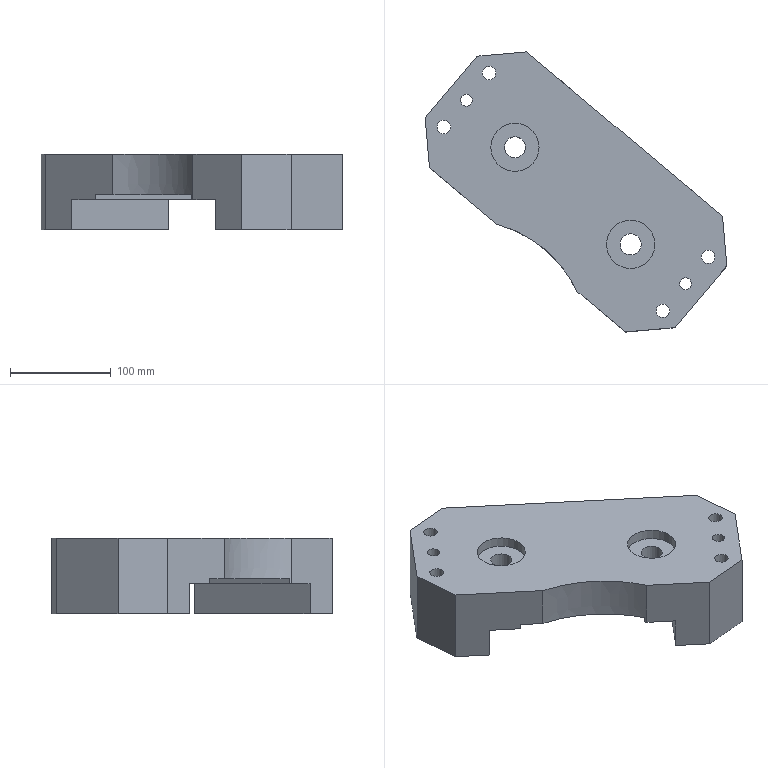Part | NX | features solid 2 | 1 solid | 52 faces | box 299.621 x 278.175 x 75 mm | volume 2327315 mm3 | plane 25 | cylinder 20 | cone 6 | spline 1 | commonest cylinder face diameters 10.579 x4 12 x4 13.5 x4 19.5 x4 21 x2 48 x2
STEP:
#1=CARTESIAN_POINT('',(632.553,521.759,95.));
#2=VERTEX_POINT('',#1);
#3=CARTESIAN_POINT('',(643.053,521.759,95.));
#4=DIRECTION('',(0.,0.,-1.));
#5=DIRECTION('',(-1.,0.,0.));
#6=AXIS2_PLACEMENT_3D('',#3,#4,#5);
#7=CIRCLE('',#6,10.5);
#8=EDGE_CURVE('',#2,#2,#7,.F.);
#9=ORIENTED_EDGE('',*,*,#8,.T.);
#10=EDGE_LOOP('',(#9));
#11=FACE_BOUND('',#10,.T.);
#12=CARTESIAN_POINT('',(588.722,477.235,95.));
#13=VERTEX_POINT('',#12);
#14=CARTESIAN_POINT('',(589.775,475.086,95.));
#15=VERTEX_POINT('',#14);
#16=CARTESIAN_POINT('',(588.722,477.235,95.));
#17=CARTESIAN_POINT('',(589.08,476.522,95.));
#18=CARTESIAN_POINT('',(589.431,475.806,95.));
#19=CARTESIAN_POINT('',(589.775,475.086,95.));
#20=B_SPLINE_CURVE_WITH_KNOTS('',3,(#16,#17,#18,#19),.UNSPECIFIED.,.F.,.F.,(4,4),(0.003786,0.006174),.UNSPECIFIED.);
#21=EDGE_CURVE('',#13,#15,#20,.T.);
#22=ORIENTED_EDGE('',*,*,#21,.F.);
#23=CARTESIAN_POINT('',(684.517,591.399,95.));
#24=VERTEX_POINT('',#23);
#25=CARTESIAN_POINT('',(594.527,484.153,95.));
#26=DIRECTION('',(-0.6428,-0.766,0.));
#27=VECTOR('',#26,1000.);
#28=LINE('',#25,#27);
#29=EDGE_CURVE('',#13,#24,#28,.F.);
#30=ORIENTED_EDGE('',*,*,#29,.T.);
#31=CARTESIAN_POINT('',(708.264,571.473,95.));
#32=VERTEX_POINT('',#31);
#33=CARTESIAN_POINT('',(577.654,681.068,95.));
#34=DIRECTION('',(-0.766,0.6428,0.));
#35=VECTOR('',#34,1000.);
#36=LINE('',#33,#35);
#37=EDGE_CURVE('',#32,#24,#36,.T.);
#38=ORIENTED_EDGE('',*,*,#37,.F.);
#39=CARTESIAN_POINT('',(611.846,456.566,95.));
#40=VERTEX_POINT('',#39);
#41=CARTESIAN_POINT('',(618.274,464.227,95.));
#42=DIRECTION('',(-0.6428,-0.766,0.));
#43=VECTOR('',#42,1000.);
#44=LINE('',#41,#43);
#45=EDGE_CURVE('',#32,#40,#44,.T.);
#46=ORIENTED_EDGE('',*,*,#45,.T.);
#47=CARTESIAN_POINT('',(481.236,566.161,95.));
#48=DIRECTION('',(0.766,-0.6428,0.));
#49=VECTOR('',#48,1000.);
#50=LINE('',#47,#49);
#51=EDGE_CURVE('',#15,#40,#50,.T.);
#52=ORIENTED_EDGE('',*,*,#51,.F.);
#53=EDGE_LOOP('',(#22,#30,#38,#46,#52));
#54=FACE_BOUND('',#53,.T.);
#55=CARTESIAN_POINT('',(487.664,573.822,95.));
#56=DIRECTION('',(0.,0.,1.));
#57=DIRECTION('',(0.08716,-0.9962,0.));
#58=AXIS2_PLACEMENT_3D('',#55,#56,#57);
#59=PLANE('',#58);
#60=ADVANCED_FACE('',(#11,#54),#59,.F.);
#61=CARTESIAN_POINT('',(589.775,475.086,140.));
#62=VERTEX_POINT('',#61);
#63=CARTESIAN_POINT('',(589.775,475.086,87.5));
#64=DIRECTION('',(0.,0.,-1.));
#65=VECTOR('',#64,1000.);
#66=LINE('',#63,#65);
#67=EDGE_CURVE('',#15,#62,#66,.F.);
#68=ORIENTED_EDGE('',*,*,#67,.F.);
#69=ORIENTED_EDGE('',*,*,#51,.T.);
#70=CARTESIAN_POINT('',(611.846,456.566,65.));
#71=VERTEX_POINT('',#70);
#72=CARTESIAN_POINT('',(611.846,456.566,95.));
#73=DIRECTION('',(0.,0.,1.));
#74=VECTOR('',#73,1000.);
#75=LINE('',#72,#74);
#76=EDGE_CURVE('',#71,#40,#75,.T.);
#77=ORIENTED_EDGE('',*,*,#76,.F.);
#78=CARTESIAN_POINT('',(637.892,434.711,65.));
#79=VERTEX_POINT('',#78);
#80=CARTESIAN_POINT('',(481.236,566.161,65.));
#81=DIRECTION('',(0.766,-0.6428,0.));
#82=VECTOR('',#81,1000.);
#83=LINE('',#80,#82);
#84=EDGE_CURVE('',#71,#79,#83,.T.);
#85=ORIENTED_EDGE('',*,*,#84,.T.);
#86=CARTESIAN_POINT('',(637.892,434.711,140.));
#87=VERTEX_POINT('',#86);
#88=CARTESIAN_POINT('',(637.892,434.711,60.));
#89=DIRECTION('',(0.,0.,-1.));
#90=VECTOR('',#89,1000.);
#91=LINE('',#88,#90);
#92=EDGE_CURVE('',#87,#79,#91,.T.);
#93=ORIENTED_EDGE('',*,*,#92,.F.);
#94=CARTESIAN_POINT('',(481.236,566.161,140.));
#95=DIRECTION('',(0.766,-0.6428,0.));
#96=VECTOR('',#95,1000.);
#97=LINE('',#94,#96);
#98=EDGE_CURVE('',#62,#87,#97,.T.);
#99=ORIENTED_EDGE('',*,*,#98,.F.);
#100=EDGE_LOOP('',(#68,#69,#77,#85,#93,#99));
#101=FACE_BOUND('',#100,.T.);
#102=CARTESIAN_POINT('',(481.236,566.161,95.));
#103=DIRECTION('',(0.6428,0.766,0.));
#104=DIRECTION('',(0.766,-0.6428,0.));
#105=AXIS2_PLACEMENT_3D('',#102,#103,#104);
#106=PLANE('',#105);
#107=ADVANCED_FACE('',(#101),#106,.F.);
#108=CARTESIAN_POINT('',(510.282,541.788,140.));
#109=VERTEX_POINT('',#108);
#110=CARTESIAN_POINT('',(510.282,541.788,100.));
#111=VERTEX_POINT('',#110);
#112=CARTESIAN_POINT('',(510.282,541.788,87.5));
#113=DIRECTION('',(0.,0.,-1.));
#114=VECTOR('',#113,1000.);
#115=LINE('',#112,#114);
#116=EDGE_CURVE('',#109,#111,#115,.T.);
#117=ORIENTED_EDGE('',*,*,#116,.F.);
#118=CARTESIAN_POINT('',(443.317,597.979,140.));
#119=VERTEX_POINT('',#118);
#120=CARTESIAN_POINT('',(481.236,566.161,140.));
#121=DIRECTION('',(0.766,-0.6428,0.));
#122=VECTOR('',#121,1000.);
#123=LINE('',#120,#122);
#124=EDGE_CURVE('',#119,#109,#123,.T.);
#125=ORIENTED_EDGE('',*,*,#124,.F.);
#126=CARTESIAN_POINT('',(443.317,597.979,65.));
#127=VERTEX_POINT('',#126);
#128=CARTESIAN_POINT('',(443.317,597.979,95.));
#129=DIRECTION('',(0.,0.,1.));
#130=VECTOR('',#129,1000.);
#131=LINE('',#128,#130);
#132=EDGE_CURVE('',#127,#119,#131,.T.);
#133=ORIENTED_EDGE('',*,*,#132,.F.);
#134=CARTESIAN_POINT('',(469.362,576.125,65.));
#135=VERTEX_POINT('',#134);
#136=CARTESIAN_POINT('',(481.236,566.161,65.));
#137=DIRECTION('',(0.766,-0.6428,0.));
#138=VECTOR('',#137,1000.);
#139=LINE('',#136,#138);
#140=EDGE_CURVE('',#127,#135,#139,.T.);
#141=ORIENTED_EDGE('',*,*,#140,.T.);
#142=CARTESIAN_POINT('',(469.362,576.125,95.));
#143=VERTEX_POINT('',#142);
#144=CARTESIAN_POINT('',(469.362,576.125,55.));
#145=DIRECTION('',(0.,0.,-1.));
#146=VECTOR('',#145,1000.);
#147=LINE('',#144,#146);
#148=EDGE_CURVE('',#143,#135,#147,.T.);
#149=ORIENTED_EDGE('',*,*,#148,.F.);
#150=CARTESIAN_POINT('',(493.109,556.198,95.));
#151=VERTEX_POINT('',#150);
#152=CARTESIAN_POINT('',(481.236,566.161,95.));
#153=DIRECTION('',(0.766,-0.6428,0.));
#154=VECTOR('',#153,1000.);
#155=LINE('',#152,#154);
#156=EDGE_CURVE('',#143,#151,#155,.T.);
#157=ORIENTED_EDGE('',*,*,#156,.T.);
#158=CARTESIAN_POINT('',(493.109,556.198,100.));
#159=VERTEX_POINT('',#158);
#160=CARTESIAN_POINT('',(493.109,556.198,100.));
#161=DIRECTION('',(0.,0.,-1.));
#162=VECTOR('',#161,1000.);
#163=LINE('',#160,#162);
#164=EDGE_CURVE('',#159,#151,#163,.T.);
#165=ORIENTED_EDGE('',*,*,#164,.F.);
#166=CARTESIAN_POINT('',(494.642,554.913,100.));
#167=DIRECTION('',(0.766,-0.6428,0.));
#168=VECTOR('',#167,1000.);
#169=LINE('',#166,#168);
#170=EDGE_CURVE('',#159,#111,#169,.T.);
#171=ORIENTED_EDGE('',*,*,#170,.T.);
#172=EDGE_LOOP('',(#117,#125,#133,#141,#149,#157,#165,#171));
#173=FACE_BOUND('',#172,.T.);
#174=CARTESIAN_POINT('',(481.236,566.161,95.));
#175=DIRECTION('',(0.6428,0.766,0.));
#176=DIRECTION('',(0.766,-0.6428,0.));
#177=AXIS2_PLACEMENT_3D('',#174,#175,#176);
#178=PLANE('',#177);
#179=ADVANCED_FACE('',(#173),#178,.F.);
#180=CARTESIAN_POINT('',(619.053,521.759,140.));
#181=VERTEX_POINT('',#180);
#182=CARTESIAN_POINT('',(643.053,521.759,140.));
#183=DIRECTION('',(0.,0.,-1.));
#184=DIRECTION('',(-1.,0.,0.));
#185=AXIS2_PLACEMENT_3D('',#182,#183,#184);
#186=CIRCLE('',#185,24.);
#187=EDGE_CURVE('',#181,#181,#186,.F.);
#188=ORIENTED_EDGE('',*,*,#187,.F.);
#189=EDGE_LOOP('',(#188));
#190=FACE_BOUND('',#189,.T.);
#191=CARTESIAN_POINT('',(504.146,618.178,140.));
#192=VERTEX_POINT('',#191);
#193=CARTESIAN_POINT('',(528.146,618.178,140.));
#194=DIRECTION('',(0.,0.,-1.));
#195=DIRECTION('',(-1.,0.,0.));
#196=AXIS2_PLACEMENT_3D('',#193,#194,#195);
#197=CIRCLE('',#196,24.);
#198=EDGE_CURVE('',#192,#192,#197,.F.);
#199=ORIENTED_EDGE('',*,*,#198,.F.);
#200=EDGE_LOOP('',(#199));
#201=FACE_BOUND('',#200,.T.);
#202=CARTESIAN_POINT('',(668.344,455.711,140.));
#203=VERTEX_POINT('',#202);
#204=CARTESIAN_POINT('',(675.094,455.711,140.));
#205=DIRECTION('',(0.,0.,-1.));
#206=DIRECTION('',(-1.,0.,0.));
#207=AXIS2_PLACEMENT_3D('',#204,#205,#206);
#208=CIRCLE('',#207,6.75);
#209=EDGE_CURVE('',#203,#203,#208,.T.);
#210=ORIENTED_EDGE('',*,*,#209,.T.);
#211=EDGE_LOOP('',(#210));
#212=FACE_BOUND('',#211,.T.);
#213=CARTESIAN_POINT('',(713.339,509.334,140.));
#214=VERTEX_POINT('',#213);
#215=CARTESIAN_POINT('',(720.089,509.334,140.));
#216=DIRECTION('',(0.,0.,-1.));
#217=DIRECTION('',(-1.,0.,0.));
#218=AXIS2_PLACEMENT_3D('',#215,#216,#217);
#219=CIRCLE('',#218,6.75);
#220=EDGE_CURVE('',#214,#214,#219,.T.);
#221=ORIENTED_EDGE('',*,*,#220,.T.);
#222=EDGE_LOOP('',(#221));
#223=FACE_BOUND('',#222,.T.);
#224=CARTESIAN_POINT('',(450.787,638.263,140.));
#225=VERTEX_POINT('',#224);
#226=CARTESIAN_POINT('',(457.537,638.263,140.));
#227=DIRECTION('',(0.,0.,-1.));
#228=DIRECTION('',(-1.,0.,0.));
#229=AXIS2_PLACEMENT_3D('',#226,#227,#228);
#230=CIRCLE('',#229,6.75);
#231=EDGE_CURVE('',#225,#225,#230,.T.);
#232=ORIENTED_EDGE('',*,*,#231,.T.);
#233=EDGE_LOOP('',(#232));
#234=FACE_BOUND('',#233,.T.);
#235=CARTESIAN_POINT('',(495.783,691.886,140.));
#236=VERTEX_POINT('',#235);
#237=CARTESIAN_POINT('',(502.533,691.886,140.));
#238=DIRECTION('',(0.,0.,-1.));
#239=DIRECTION('',(-1.,0.,0.));
#240=AXIS2_PLACEMENT_3D('',#237,#238,#239);
#241=CIRCLE('',#240,6.75);
#242=EDGE_CURVE('',#236,#236,#241,.T.);
#243=ORIENTED_EDGE('',*,*,#242,.T.);
#244=EDGE_LOOP('',(#243));
#245=FACE_BOUND('',#244,.T.);
#246=CARTESIAN_POINT('',(691.592,482.523,140.));
#247=VERTEX_POINT('',#246);
#248=CARTESIAN_POINT('',(697.592,482.523,140.));
#249=DIRECTION('',(0.,0.,-1.));
#250=DIRECTION('',(-1.,0.,0.));
#251=AXIS2_PLACEMENT_3D('',#248,#249,#250);
#252=CIRCLE('',#251,6.);
#253=EDGE_CURVE('',#247,#247,#252,.T.);
#254=ORIENTED_EDGE('',*,*,#253,.T.);
#255=EDGE_LOOP('',(#254));
#256=FACE_BOUND('',#255,.T.);
#257=CARTESIAN_POINT('',(474.035,665.075,140.));
#258=VERTEX_POINT('',#257);
#259=CARTESIAN_POINT('',(480.035,665.075,140.));
#260=DIRECTION('',(0.,0.,-1.));
#261=DIRECTION('',(-1.,0.,0.));
#262=AXIS2_PLACEMENT_3D('',#259,#260,#261);
#263=CIRCLE('',#262,6.);
#264=EDGE_CURVE('',#258,#258,#263,.T.);
#265=ORIENTED_EDGE('',*,*,#264,.T.);
#266=EDGE_LOOP('',(#265));
#267=FACE_BOUND('',#266,.T.);
#268=ORIENTED_EDGE('',*,*,#124,.T.);
#269=CARTESIAN_POINT('',(510.282,541.788,140.));
#270=CARTESIAN_POINT('',(518.848,539.431,140.));
#271=CARTESIAN_POINT('',(535.724,532.766,140.));
#272=CARTESIAN_POINT('',(554.078,520.489,140.));
#273=CARTESIAN_POINT('',(567.262,508.143,140.));
#274=CARTESIAN_POINT('',(575.948,498.015,140.));
#275=CARTESIAN_POINT('',(583.527,487.052,140.));
#276=CARTESIAN_POINT('',(587.84,479.13,140.));
#277=CARTESIAN_POINT('',(589.775,475.086,140.));
#278=B_SPLINE_CURVE_WITH_KNOTS('',3,(#269,#270,#271,#272,#273,#274,#275,#276,#277),.UNSPECIFIED.,.F.,.F.,(4,1,1,1,1,1,4),(0.03089,0.0575,0.0841,0.09741,0.1107,0.124,0.1373),.UNSPECIFIED.);
#279=EDGE_CURVE('',#109,#62,#278,.T.);
#280=ORIENTED_EDGE('',*,*,#279,.T.);
#281=ORIENTED_EDGE('',*,*,#98,.T.);
#282=CARTESIAN_POINT('',(687.201,439.025,140.));
#283=VERTEX_POINT('',#282);
#284=CARTESIAN_POINT('',(522.015,424.573,140.));
#285=DIRECTION('',(-0.9962,-0.08716,0.));
#286=VECTOR('',#285,1000.);
#287=LINE('',#284,#286);
#288=EDGE_CURVE('',#283,#87,#287,.T.);
#289=ORIENTED_EDGE('',*,*,#288,.F.);
#290=CARTESIAN_POINT('',(738.624,500.309,140.));
#291=VERTEX_POINT('',#290);
#292=CARTESIAN_POINT('',(671.131,419.874,140.));
#293=DIRECTION('',(-0.6428,-0.766,0.));
#294=VECTOR('',#293,1000.);
#295=LINE('',#292,#294);
#296=EDGE_CURVE('',#291,#283,#295,.T.);
#297=ORIENTED_EDGE('',*,*,#296,.F.);
#298=CARTESIAN_POINT('',(734.31,549.618,140.));
#299=VERTEX_POINT('',#298);
#300=CARTESIAN_POINT('',(732.8,566.876,140.));
#301=DIRECTION('',(0.08716,-0.9962,0.));
#302=VECTOR('',#301,1000.);
#303=LINE('',#300,#302);
#304=EDGE_CURVE('',#299,#291,#303,.T.);
#305=ORIENTED_EDGE('',*,*,#304,.F.);
#306=CARTESIAN_POINT('',(539.735,712.886,140.));
#307=VERTEX_POINT('',#306);
#308=CARTESIAN_POINT('',(577.654,681.068,140.));
#309=DIRECTION('',(-0.766,0.6428,0.));
#310=VECTOR('',#309,1000.);
#311=LINE('',#308,#310);
#312=EDGE_CURVE('',#299,#307,#311,.T.);
#313=ORIENTED_EDGE('',*,*,#312,.T.);
#314=CARTESIAN_POINT('',(490.426,708.572,140.));
#315=VERTEX_POINT('',#314);
#316=CARTESIAN_POINT('',(447.808,704.844,140.));
#317=DIRECTION('',(-0.9962,-0.08716,0.));
#318=VECTOR('',#317,1000.);
#319=LINE('',#316,#318);
#320=EDGE_CURVE('',#315,#307,#319,.F.);
#321=ORIENTED_EDGE('',*,*,#320,.F.);
#322=CARTESIAN_POINT('',(439.003,647.289,140.));
#323=VERTEX_POINT('',#322);
#324=CARTESIAN_POINT('',(422.933,628.137,140.));
#325=DIRECTION('',(-0.6428,-0.766,0.));
#326=VECTOR('',#325,1000.);
#327=LINE('',#324,#326);
#328=EDGE_CURVE('',#315,#323,#327,.T.);
#329=ORIENTED_EDGE('',*,*,#328,.T.);
#330=CARTESIAN_POINT('',(443.902,591.287,140.));
#331=DIRECTION('',(0.08716,-0.9962,0.));
#332=VECTOR('',#331,1000.);
#333=LINE('',#330,#332);
#334=EDGE_CURVE('',#119,#323,#333,.F.);
#335=ORIENTED_EDGE('',*,*,#334,.F.);
#336=EDGE_LOOP('',(#268,#280,#281,#289,#297,#305,#313,#321,#329,#335));
#337=FACE_BOUND('',#336,.T.);
#338=CARTESIAN_POINT('',(487.664,573.822,140.));
#339=DIRECTION('',(0.,0.,1.));
#340=DIRECTION('',(0.08716,-0.9962,0.));
#341=AXIS2_PLACEMENT_3D('',#338,#339,#340);
#342=PLANE('',#341);
#343=ADVANCED_FACE('',(#190,#201,#212,#223,#234,#245,#256,#267,#337),#342,.T.);
#344=ORIENTED_EDGE('',*,*,#29,.F.);
#345=CARTESIAN_POINT('',(588.722,477.235,100.));
#346=VERTEX_POINT('',#345);
#347=CARTESIAN_POINT('',(588.722,477.235,87.5));
#348=DIRECTION('',(0.,0.,-1.));
#349=VECTOR('',#348,1000.);
#350=LINE('',#347,#349);
#351=EDGE_CURVE('',#13,#346,#350,.F.);
#352=ORIENTED_EDGE('',*,*,#351,.T.);
#353=CARTESIAN_POINT('',(684.517,591.399,100.));
#354=VERTEX_POINT('',#353);
#355=CARTESIAN_POINT('',(652.378,553.097,100.));
#356=DIRECTION('',(0.6428,0.766,0.));
#357=VECTOR('',#356,1000.);
#358=LINE('',#355,#357);
#359=EDGE_CURVE('',#354,#346,#358,.F.);
#360=ORIENTED_EDGE('',*,*,#359,.F.);
#361=CARTESIAN_POINT('',(684.517,591.399,100.));
#362=DIRECTION('',(0.,0.,1.));
#363=VECTOR('',#362,1000.);
#364=LINE('',#361,#363);
#365=EDGE_CURVE('',#354,#24,#364,.F.);
#366=ORIENTED_EDGE('',*,*,#365,.T.);
#367=EDGE_LOOP('',(#344,#352,#360,#366));
#368=FACE_BOUND('',#367,.T.);
#369=CARTESIAN_POINT('',(652.378,553.097,100.));
#370=DIRECTION('',(0.766,-0.6428,0.));
#371=DIRECTION('',(-0.6428,-0.766,0.));
#372=AXIS2_PLACEMENT_3D('',#369,#370,#371);
#373=PLANE('',#372);
#374=ADVANCED_FACE('',(#368),#373,.F.);
#375=CARTESIAN_POINT('',(510.282,541.788,100.));
#376=CARTESIAN_POINT('',(514.467,540.637,100.));
#377=CARTESIAN_POINT('',(522.696,537.916,100.));
#378=CARTESIAN_POINT('',(534.726,532.472,100.));
#379=CARTESIAN_POINT('',(546.029,525.84,100.));
#380=CARTESIAN_POINT('',(556.487,518.125,100.));
#381=CARTESIAN_POINT('',(566.167,509.258,100.));
#382=CARTESIAN_POINT('',(577.791,496.068,100.));
#383=CARTESIAN_POINT('',(584.787,485.085,100.));
#384=CARTESIAN_POINT('',(588.722,477.235,100.));
#385=B_SPLINE_CURVE_WITH_KNOTS('',3,(#375,#376,#377,#378,#379,#380,#381,#382,#383,#384),.UNSPECIFIED.,.F.,.F.,(4,1,1,1,1,1,1,4),(0.0186,0.03162,0.04464,0.05766,0.07067,0.08369,0.09671,0.1227),.UNSPECIFIED.);
#386=EDGE_CURVE('',#111,#346,#385,.T.);
#387=ORIENTED_EDGE('',*,*,#386,.F.);
#388=ORIENTED_EDGE('',*,*,#170,.F.);
#389=CARTESIAN_POINT('',(589.528,671.105,100.));
#390=VERTEX_POINT('',#389);
#391=CARTESIAN_POINT('',(557.388,632.803,100.));
#392=DIRECTION('',(-0.6428,-0.766,0.));
#393=VECTOR('',#392,1000.);
#394=LINE('',#391,#393);
#395=EDGE_CURVE('',#390,#159,#394,.T.);
#396=ORIENTED_EDGE('',*,*,#395,.F.);
#397=CARTESIAN_POINT('',(577.654,681.068,100.));
#398=DIRECTION('',(0.766,-0.6428,0.));
#399=VECTOR('',#398,1000.);
#400=LINE('',#397,#399);
#401=EDGE_CURVE('',#390,#354,#400,.T.);
#402=ORIENTED_EDGE('',*,*,#401,.T.);
#403=ORIENTED_EDGE('',*,*,#359,.T.);
#404=EDGE_LOOP('',(#387,#388,#396,#402,#403));
#405=FACE_BOUND('',#404,.T.);
#406=CARTESIAN_POINT('',(558.92,631.517,100.));
#407=DIRECTION('',(0.,0.,1.));
#408=DIRECTION('',(-1.,0.,0.));
#409=AXIS2_PLACEMENT_3D('',#406,#407,#408);
#410=PLANE('',#409);
#411=ADVANCED_FACE('',(#405),#410,.F.);
#412=CARTESIAN_POINT('',(517.646,618.178,95.));
#413=VERTEX_POINT('',#412);
#414=CARTESIAN_POINT('',(528.146,618.178,95.));
#415=DIRECTION('',(0.,0.,-1.));
#416=DIRECTION('',(-1.,0.,0.));
#417=AXIS2_PLACEMENT_3D('',#414,#415,#416);
#418=CIRCLE('',#417,10.5);
#419=EDGE_CURVE('',#413,#413,#418,.F.);
#420=ORIENTED_EDGE('',*,*,#419,.T.);
#421=EDGE_LOOP('',(#420));
#422=FACE_BOUND('',#421,.T.);
#423=CARTESIAN_POINT('',(589.528,671.105,95.));
#424=VERTEX_POINT('',#423);
#425=CARTESIAN_POINT('',(499.537,563.859,95.));
#426=DIRECTION('',(-0.6428,-0.766,0.));
#427=VECTOR('',#426,1000.);
#428=LINE('',#425,#427);
#429=EDGE_CURVE('',#424,#151,#428,.T.);
#430=ORIENTED_EDGE('',*,*,#429,.T.);
#431=ORIENTED_EDGE('',*,*,#156,.F.);
#432=CARTESIAN_POINT('',(565.78,691.031,95.));
#433=VERTEX_POINT('',#432);
#434=CARTESIAN_POINT('',(475.79,583.785,95.));
#435=DIRECTION('',(-0.6428,-0.766,0.));
#436=VECTOR('',#435,1000.);
#437=LINE('',#434,#436);
#438=EDGE_CURVE('',#433,#143,#437,.T.);
#439=ORIENTED_EDGE('',*,*,#438,.F.);
#440=CARTESIAN_POINT('',(577.654,681.068,95.));
#441=DIRECTION('',(-0.766,0.6428,0.));
#442=VECTOR('',#441,1000.);
#443=LINE('',#440,#442);
#444=EDGE_CURVE('',#424,#433,#443,.T.);
#445=ORIENTED_EDGE('',*,*,#444,.F.);
#446=EDGE_LOOP('',(#430,#431,#439,#445));
#447=FACE_BOUND('',#446,.T.);
#448=CARTESIAN_POINT('',(487.664,573.822,95.));
#449=DIRECTION('',(0.,0.,1.));
#450=DIRECTION('',(0.08716,-0.9962,0.));
#451=AXIS2_PLACEMENT_3D('',#448,#449,#450);
#452=PLANE('',#451);
#453=ADVANCED_FACE('',(#422,#447),#452,.F.);
#454=CARTESIAN_POINT('',(667.053,521.759,130.));
#455=VERTEX_POINT('',#454);
#456=CARTESIAN_POINT('',(643.053,521.759,130.));
#457=DIRECTION('',(0.,0.,1.));
#458=DIRECTION('',(1.,0.,0.));
#459=AXIS2_PLACEMENT_3D('',#456,#457,#458);
#460=CIRCLE('',#459,24.);
#461=EDGE_CURVE('',#455,#455,#460,.F.);
#462=ORIENTED_EDGE('',*,*,#461,.F.);
#463=EDGE_LOOP('',(#462));
#464=FACE_BOUND('',#463,.T.);
#465=CARTESIAN_POINT('',(653.553,521.759,130.));
#466=VERTEX_POINT('',#465);
#467=CARTESIAN_POINT('',(643.053,521.759,130.));
#468=DIRECTION('',(0.,0.,1.));
#469=DIRECTION('',(1.,0.,0.));
#470=AXIS2_PLACEMENT_3D('',#467,#468,#469);
#471=CIRCLE('',#470,10.5);
#472=EDGE_CURVE('',#466,#466,#471,.F.);
#473=ORIENTED_EDGE('',*,*,#472,.T.);
#474=EDGE_LOOP('',(#473));
#475=FACE_BOUND('',#474,.T.);
#476=CARTESIAN_POINT('',(528.146,618.178,130.));
#477=DIRECTION('',(0.,0.,-1.));
#478=DIRECTION('',(-1.,0.,0.));
#479=AXIS2_PLACEMENT_3D('',#476,#477,#478);
#480=PLANE('',#479);
#481=ADVANCED_FACE('',(#464,#475),#480,.F.);
#482=CARTESIAN_POINT('',(552.146,618.178,130.));
#483=VERTEX_POINT('',#482);
#484=CARTESIAN_POINT('',(528.146,618.178,130.));
#485=DIRECTION('',(0.,0.,1.));
#486=DIRECTION('',(1.,0.,0.));
#487=AXIS2_PLACEMENT_3D('',#484,#485,#486);
#488=CIRCLE('',#487,24.);
#489=EDGE_CURVE('',#483,#483,#488,.T.);
#490=ORIENTED_EDGE('',*,*,#489,.T.);
#491=EDGE_LOOP('',(#490));
#492=FACE_BOUND('',#491,.T.);
#493=CARTESIAN_POINT('',(538.646,618.178,130.));
#494=VERTEX_POINT('',#493);
#495=CARTESIAN_POINT('',(528.146,618.178,130.));
#496=DIRECTION('',(0.,0.,1.));
#497=DIRECTION('',(1.,0.,0.));
#498=AXIS2_PLACEMENT_3D('',#495,#496,#497);
#499=CIRCLE('',#498,10.5);
#500=EDGE_CURVE('',#494,#494,#499,.F.);
#501=ORIENTED_EDGE('',*,*,#500,.T.);
#502=EDGE_LOOP('',(#501));
#503=FACE_BOUND('',#502,.T.);
#504=CARTESIAN_POINT('',(528.146,618.178,130.));
#505=DIRECTION('',(0.,0.,-1.));
#506=DIRECTION('',(-1.,0.,0.));
#507=AXIS2_PLACEMENT_3D('',#504,#505,#506);
#508=PLANE('',#507);
#509=ADVANCED_FACE('',(#492,#503),#508,.F.);
#510=CARTESIAN_POINT('',(589.528,671.105,95.));
#511=DIRECTION('',(0.,0.,-1.));
#512=VECTOR('',#511,1000.);
#513=LINE('',#510,#512);
#514=EDGE_CURVE('',#390,#424,#513,.T.);
#515=ORIENTED_EDGE('',*,*,#514,.T.);
#516=ORIENTED_EDGE('',*,*,#444,.T.);
#517=CARTESIAN_POINT('',(565.78,691.031,65.));
#518=VERTEX_POINT('',#517);
#519=CARTESIAN_POINT('',(565.78,691.031,95.));
#520=DIRECTION('',(0.,0.,-1.));
#521=VECTOR('',#520,1000.);
#522=LINE('',#519,#521);
#523=EDGE_CURVE('',#433,#518,#522,.T.);
#524=ORIENTED_EDGE('',*,*,#523,.T.);
#525=CARTESIAN_POINT('',(539.735,712.886,65.));
#526=VERTEX_POINT('',#525);
#527=CARTESIAN_POINT('',(577.654,681.068,65.));
#528=DIRECTION('',(-0.766,0.6428,0.));
#529=VECTOR('',#528,1000.);
#530=LINE('',#527,#529);
#531=EDGE_CURVE('',#518,#526,#530,.T.);
#532=ORIENTED_EDGE('',*,*,#531,.T.);
#533=CARTESIAN_POINT('',(539.735,712.886,95.));
#534=DIRECTION('',(0.,0.,-1.));
#535=VECTOR('',#534,1000.);
#536=LINE('',#533,#535);
#537=EDGE_CURVE('',#307,#526,#536,.T.);
#538=ORIENTED_EDGE('',*,*,#537,.F.);
#539=ORIENTED_EDGE('',*,*,#312,.F.);
#540=CARTESIAN_POINT('',(734.31,549.618,65.));
#541=VERTEX_POINT('',#540);
#542=CARTESIAN_POINT('',(734.31,549.618,135.));
#543=DIRECTION('',(0.,0.,1.));
#544=VECTOR('',#543,1000.);
#545=LINE('',#542,#544);
#546=EDGE_CURVE('',#541,#299,#545,.T.);
#547=ORIENTED_EDGE('',*,*,#546,.F.);
#548=CARTESIAN_POINT('',(708.264,571.473,65.));
#549=VERTEX_POINT('',#548);
#550=CARTESIAN_POINT('',(577.654,681.068,65.));
#551=DIRECTION('',(-0.766,0.6428,0.));
#552=VECTOR('',#551,1000.);
#553=LINE('',#550,#552);
#554=EDGE_CURVE('',#541,#549,#553,.T.);
#555=ORIENTED_EDGE('',*,*,#554,.T.);
#556=CARTESIAN_POINT('',(708.264,571.473,55.));
#557=DIRECTION('',(0.,0.,1.));
#558=VECTOR('',#557,1000.);
#559=LINE('',#556,#558);
#560=EDGE_CURVE('',#549,#32,#559,.T.);
#561=ORIENTED_EDGE('',*,*,#560,.T.);
#562=ORIENTED_EDGE('',*,*,#37,.T.);
#563=ORIENTED_EDGE('',*,*,#365,.F.);
#564=ORIENTED_EDGE('',*,*,#401,.F.);
#565=EDGE_LOOP('',(#515,#516,#524,#532,#538,#539,#547,#555,#561,#562,#563,#564));
#566=FACE_BOUND('',#565,.T.);
#567=CARTESIAN_POINT('',(577.654,681.068,95.));
#568=DIRECTION('',(-0.6428,-0.766,0.));
#569=DIRECTION('',(-0.766,0.6428,0.));
#570=AXIS2_PLACEMENT_3D('',#567,#568,#569);
#571=PLANE('',#570);
#572=ADVANCED_FACE('',(#566),#571,.F.);
#573=CARTESIAN_POINT('',(509.016,645.791,65.));
#574=VERTEX_POINT('',#573);
#575=CARTESIAN_POINT('',(503.016,645.791,65.));
#576=DIRECTION('',(0.,0.,1.));
#577=DIRECTION('',(1.,0.,0.));
#578=AXIS2_PLACEMENT_3D('',#575,#576,#577);
#579=CIRCLE('',#578,6.);
#580=EDGE_CURVE('',#574,#574,#579,.T.);
#581=ORIENTED_EDGE('',*,*,#580,.T.);
#582=EDGE_LOOP('',(#581));
#583=FACE_BOUND('',#582,.T.);
#584=CARTESIAN_POINT('',(543.659,687.923,65.));
#585=VERTEX_POINT('',#584);
#586=CARTESIAN_POINT('',(538.37,687.923,65.));
#587=DIRECTION('',(0.,0.,1.));
#588=DIRECTION('',(1.,0.,0.));
#589=AXIS2_PLACEMENT_3D('',#586,#587,#588);
#590=CIRCLE('',#589,5.29);
#591=EDGE_CURVE('',#585,#585,#590,.T.);
#592=ORIENTED_EDGE('',*,*,#591,.T.);
#593=EDGE_LOOP('',(#592));
#594=FACE_BOUND('',#593,.T.);
#595=CARTESIAN_POINT('',(472.953,603.658,65.));
#596=VERTEX_POINT('',#595);
#597=CARTESIAN_POINT('',(467.663,603.658,65.));
#598=DIRECTION('',(0.,0.,1.));
#599=DIRECTION('',(1.,0.,0.));
#600=AXIS2_PLACEMENT_3D('',#597,#598,#599);
#601=CIRCLE('',#600,5.29);
#602=EDGE_CURVE('',#596,#596,#601,.T.);
#603=ORIENTED_EDGE('',*,*,#602,.T.);
#604=EDGE_LOOP('',(#603));
#605=FACE_BOUND('',#604,.T.);
#606=CARTESIAN_POINT('',(474.035,665.075,65.));
#607=VERTEX_POINT('',#606);
#608=CARTESIAN_POINT('',(480.035,665.075,65.));
#609=DIRECTION('',(0.,0.,-1.));
#610=DIRECTION('',(-1.,0.,0.));
#611=AXIS2_PLACEMENT_3D('',#608,#609,#610);
#612=CIRCLE('',#611,6.);
#613=EDGE_CURVE('',#607,#607,#612,.T.);
#614=ORIENTED_EDGE('',*,*,#613,.F.);
#615=EDGE_LOOP('',(#614));
#616=FACE_BOUND('',#615,.T.);
#617=CARTESIAN_POINT('',(492.783,691.886,65.));
#618=VERTEX_POINT('',#617);
#619=CARTESIAN_POINT('',(502.533,691.886,65.));
#620=DIRECTION('',(0.,0.,-1.));
#621=DIRECTION('',(-1.,0.,0.));
#622=AXIS2_PLACEMENT_3D('',#619,#620,#621);
#623=CIRCLE('',#622,9.75);
#624=EDGE_CURVE('',#618,#618,#623,.T.);
#625=ORIENTED_EDGE('',*,*,#624,.F.);
#626=EDGE_LOOP('',(#625));
#627=FACE_BOUND('',#626,.T.);
#628=CARTESIAN_POINT('',(447.787,638.263,65.));
#629=VERTEX_POINT('',#628);
#630=CARTESIAN_POINT('',(457.537,638.263,65.));
#631=DIRECTION('',(0.,0.,-1.));
#632=DIRECTION('',(-1.,0.,0.));
#633=AXIS2_PLACEMENT_3D('',#630,#631,#632);
#634=CIRCLE('',#633,9.75);
#635=EDGE_CURVE('',#629,#629,#634,.T.);
#636=ORIENTED_EDGE('',*,*,#635,.F.);
#637=EDGE_LOOP('',(#636));
#638=FACE_BOUND('',#637,.T.);
#639=ORIENTED_EDGE('',*,*,#531,.F.);
#640=CARTESIAN_POINT('',(475.79,583.785,65.));
#641=DIRECTION('',(-0.6428,-0.766,0.));
#642=VECTOR('',#641,1000.);
#643=LINE('',#640,#642);
#644=EDGE_CURVE('',#518,#135,#643,.T.);
#645=ORIENTED_EDGE('',*,*,#644,.T.);
#646=ORIENTED_EDGE('',*,*,#140,.F.);
#647=CARTESIAN_POINT('',(439.003,647.289,65.));
#648=VERTEX_POINT('',#647);
#649=CARTESIAN_POINT('',(443.317,597.979,65.));
#650=DIRECTION('',(-0.08716,0.9962,0.));
#651=VECTOR('',#650,1000.);
#652=LINE('',#649,#651);
#653=EDGE_CURVE('',#648,#127,#652,.F.);
#654=ORIENTED_EDGE('',*,*,#653,.F.);
#655=CARTESIAN_POINT('',(490.426,708.572,65.));
#656=VERTEX_POINT('',#655);
#657=CARTESIAN_POINT('',(422.933,628.137,65.));
#658=DIRECTION('',(-0.6428,-0.766,0.));
#659=VECTOR('',#658,1000.);
#660=LINE('',#657,#659);
#661=EDGE_CURVE('',#656,#648,#660,.T.);
#662=ORIENTED_EDGE('',*,*,#661,.F.);
#663=CARTESIAN_POINT('',(497.47,709.188,65.));
#664=DIRECTION('',(0.9962,0.08716,0.));
#665=VECTOR('',#664,1000.);
#666=LINE('',#663,#665);
#667=EDGE_CURVE('',#526,#656,#666,.F.);
#668=ORIENTED_EDGE('',*,*,#667,.F.);
#669=EDGE_LOOP('',(#639,#645,#646,#654,#662,#668));
#670=FACE_BOUND('',#669,.T.);
#671=CARTESIAN_POINT('',(487.664,573.822,65.));
#672=DIRECTION('',(0.,0.,1.));
#673=DIRECTION('',(0.08716,-0.9962,0.));
#674=AXIS2_PLACEMENT_3D('',#671,#672,#673);
#675=PLANE('',#674);
#676=ADVANCED_FACE('',(#583,#594,#605,#616,#627,#638,#670),#675,.F.);
#677=CARTESIAN_POINT('',(680.61,501.806,65.));
#678=VERTEX_POINT('',#677);
#679=CARTESIAN_POINT('',(674.61,501.806,65.));
#680=DIRECTION('',(0.,0.,1.));
#681=DIRECTION('',(1.,0.,0.));
#682=AXIS2_PLACEMENT_3D('',#679,#680,#681);
#683=CIRCLE('',#682,6.);
#684=EDGE_CURVE('',#678,#678,#683,.T.);
#685=ORIENTED_EDGE('',*,*,#684,.T.);
#686=EDGE_LOOP('',(#685));
#687=FACE_BOUND('',#686,.T.);
#688=CARTESIAN_POINT('',(715.253,543.939,65.));
#689=VERTEX_POINT('',#688);
#690=CARTESIAN_POINT('',(709.964,543.939,65.));
#691=DIRECTION('',(0.,0.,1.));
#692=DIRECTION('',(1.,0.,0.));
#693=AXIS2_PLACEMENT_3D('',#690,#691,#692);
#694=CIRCLE('',#693,5.29);
#695=EDGE_CURVE('',#689,#689,#694,.T.);
#696=ORIENTED_EDGE('',*,*,#695,.T.);
#697=EDGE_LOOP('',(#696));
#698=FACE_BOUND('',#697,.T.);
#699=CARTESIAN_POINT('',(644.547,459.674,65.));
#700=VERTEX_POINT('',#699);
#701=CARTESIAN_POINT('',(639.257,459.674,65.));
#702=DIRECTION('',(0.,0.,1.));
#703=DIRECTION('',(1.,0.,0.));
#704=AXIS2_PLACEMENT_3D('',#701,#702,#703);
#705=CIRCLE('',#704,5.29);
#706=EDGE_CURVE('',#700,#700,#705,.T.);
#707=ORIENTED_EDGE('',*,*,#706,.T.);
#708=EDGE_LOOP('',(#707));
#709=FACE_BOUND('',#708,.T.);
#710=CARTESIAN_POINT('',(691.592,482.523,65.));
#711=VERTEX_POINT('',#710);
#712=CARTESIAN_POINT('',(697.592,482.523,65.));
#713=DIRECTION('',(0.,0.,-1.));
#714=DIRECTION('',(-1.,0.,0.));
#715=AXIS2_PLACEMENT_3D('',#712,#713,#714);
#716=CIRCLE('',#715,6.);
#717=EDGE_CURVE('',#711,#711,#716,.T.);
#718=ORIENTED_EDGE('',*,*,#717,.F.);
#719=EDGE_LOOP('',(#718));
#720=FACE_BOUND('',#719,.T.);
#721=CARTESIAN_POINT('',(710.339,509.334,65.));
#722=VERTEX_POINT('',#721);
#723=CARTESIAN_POINT('',(720.089,509.334,65.));
#724=DIRECTION('',(0.,0.,-1.));
#725=DIRECTION('',(-1.,0.,0.));
#726=AXIS2_PLACEMENT_3D('',#723,#724,#725);
#727=CIRCLE('',#726,9.75);
#728=EDGE_CURVE('',#722,#722,#727,.T.);
#729=ORIENTED_EDGE('',*,*,#728,.F.);
#730=EDGE_LOOP('',(#729));
#731=FACE_BOUND('',#730,.T.);
#732=CARTESIAN_POINT('',(665.344,455.711,65.));
#733=VERTEX_POINT('',#732);
#734=CARTESIAN_POINT('',(675.094,455.711,65.));
#735=DIRECTION('',(0.,0.,-1.));
#736=DIRECTION('',(-1.,0.,0.));
#737=AXIS2_PLACEMENT_3D('',#734,#735,#736);
#738=CIRCLE('',#737,9.75);
#739=EDGE_CURVE('',#733,#733,#738,.T.);
#740=ORIENTED_EDGE('',*,*,#739,.F.);
#741=EDGE_LOOP('',(#740));
#742=FACE_BOUND('',#741,.T.);
#743=CARTESIAN_POINT('',(738.624,500.309,65.));
#744=VERTEX_POINT('',#743);
#745=CARTESIAN_POINT('',(687.201,439.025,65.));
#746=VERTEX_POINT('',#745);
#747=CARTESIAN_POINT('',(671.131,419.874,65.));
#748=DIRECTION('',(-0.6428,-0.766,0.));
#749=VECTOR('',#748,1000.);
#750=LINE('',#747,#749);
#751=EDGE_CURVE('',#744,#746,#750,.T.);
#752=ORIENTED_EDGE('',*,*,#751,.T.);
#753=CARTESIAN_POINT('',(680.157,438.409,65.));
#754=DIRECTION('',(0.9962,0.08716,0.));
#755=VECTOR('',#754,1000.);
#756=LINE('',#753,#755);
#757=EDGE_CURVE('',#79,#746,#756,.T.);
#758=ORIENTED_EDGE('',*,*,#757,.F.);
#759=ORIENTED_EDGE('',*,*,#84,.F.);
#760=CARTESIAN_POINT('',(618.274,464.227,65.));
#761=DIRECTION('',(-0.6428,-0.766,0.));
#762=VECTOR('',#761,1000.);
#763=LINE('',#760,#762);
#764=EDGE_CURVE('',#549,#71,#763,.T.);
#765=ORIENTED_EDGE('',*,*,#764,.F.);
#766=ORIENTED_EDGE('',*,*,#554,.F.);
#767=CARTESIAN_POINT('',(734.31,549.618,65.));
#768=DIRECTION('',(-0.08716,0.9962,0.));
#769=VECTOR('',#768,1000.);
#770=LINE('',#767,#769);
#771=EDGE_CURVE('',#744,#541,#770,.T.);
#772=ORIENTED_EDGE('',*,*,#771,.F.);
#773=EDGE_LOOP('',(#752,#758,#759,#765,#766,#772));
#774=FACE_BOUND('',#773,.T.);
#775=CARTESIAN_POINT('',(487.664,573.822,65.));
#776=DIRECTION('',(0.,0.,1.));
#777=DIRECTION('',(0.08716,-0.9962,0.));
#778=AXIS2_PLACEMENT_3D('',#775,#776,#777);
#779=PLANE('',#778);
#780=ADVANCED_FACE('',(#687,#698,#709,#720,#731,#742,#774),#779,.F.);
#781=ORIENTED_EDGE('',*,*,#76,.T.);
#782=ORIENTED_EDGE('',*,*,#45,.F.);
#783=ORIENTED_EDGE('',*,*,#560,.F.);
#784=ORIENTED_EDGE('',*,*,#764,.T.);
#785=EDGE_LOOP('',(#781,#782,#783,#784));
#786=FACE_BOUND('',#785,.T.);
#787=CARTESIAN_POINT('',(663.269,517.85,55.));
#788=DIRECTION('',(0.766,-0.6428,0.));
#789=DIRECTION('',(-0.6428,-0.766,0.));
#790=AXIS2_PLACEMENT_3D('',#787,#788,#789);
#791=PLANE('',#790);
#792=ADVANCED_FACE('',(#786),#791,.F.);
#793=ORIENTED_EDGE('',*,*,#148,.T.);
#794=ORIENTED_EDGE('',*,*,#644,.F.);
#795=ORIENTED_EDGE('',*,*,#523,.F.);
#796=ORIENTED_EDGE('',*,*,#438,.T.);
#797=EDGE_LOOP('',(#793,#794,#795,#796));
#798=FACE_BOUND('',#797,.T.);
#799=CARTESIAN_POINT('',(527.213,645.069,55.));
#800=DIRECTION('',(0.766,-0.6428,0.));
#801=DIRECTION('',(-0.6428,-0.766,0.));
#802=AXIS2_PLACEMENT_3D('',#799,#800,#801);
#803=PLANE('',#802);
#804=ADVANCED_FACE('',(#798),#803,.T.);
#805=ORIENTED_EDGE('',*,*,#296,.T.);
#806=CARTESIAN_POINT('',(687.201,439.025,95.));
#807=DIRECTION('',(0.,0.,1.));
#808=VECTOR('',#807,1000.);
#809=LINE('',#806,#808);
#810=EDGE_CURVE('',#746,#283,#809,.T.);
#811=ORIENTED_EDGE('',*,*,#810,.F.);
#812=ORIENTED_EDGE('',*,*,#751,.F.);
#813=CARTESIAN_POINT('',(738.624,500.309,95.));
#814=DIRECTION('',(0.,0.,-1.));
#815=VECTOR('',#814,1000.);
#816=LINE('',#813,#815);
#817=EDGE_CURVE('',#291,#744,#816,.T.);
#818=ORIENTED_EDGE('',*,*,#817,.F.);
#819=EDGE_LOOP('',(#805,#811,#812,#818));
#820=FACE_BOUND('',#819,.T.);
#821=CARTESIAN_POINT('',(671.131,419.874,95.));
#822=DIRECTION('',(0.766,-0.6428,0.));
#823=DIRECTION('',(-0.6428,-0.766,0.));
#824=AXIS2_PLACEMENT_3D('',#821,#822,#823);
#825=PLANE('',#824);
#826=ADVANCED_FACE('',(#820),#825,.T.);
#827=ORIENTED_EDGE('',*,*,#661,.T.);
#828=CARTESIAN_POINT('',(439.003,647.289,95.));
#829=DIRECTION('',(0.,0.,1.));
#830=VECTOR('',#829,1000.);
#831=LINE('',#828,#830);
#832=EDGE_CURVE('',#323,#648,#831,.F.);
#833=ORIENTED_EDGE('',*,*,#832,.F.);
#834=ORIENTED_EDGE('',*,*,#328,.F.);
#835=CARTESIAN_POINT('',(490.426,708.572,95.));
#836=DIRECTION('',(0.,0.,-1.));
#837=VECTOR('',#836,1000.);
#838=LINE('',#835,#837);
#839=EDGE_CURVE('',#656,#315,#838,.F.);
#840=ORIENTED_EDGE('',*,*,#839,.F.);
#841=EDGE_LOOP('',(#827,#833,#834,#840));
#842=FACE_BOUND('',#841,.T.);
#843=CARTESIAN_POINT('',(422.933,628.137,95.));
#844=DIRECTION('',(0.766,-0.6428,0.));
#845=DIRECTION('',(-0.6428,-0.766,0.));
#846=AXIS2_PLACEMENT_3D('',#843,#844,#845);
#847=PLANE('',#846);
#848=ADVANCED_FACE('',(#842),#847,.F.);
#849=ORIENTED_EDGE('',*,*,#757,.T.);
#850=ORIENTED_EDGE('',*,*,#810,.T.);
#851=ORIENTED_EDGE('',*,*,#288,.T.);
#852=ORIENTED_EDGE('',*,*,#92,.T.);
#853=EDGE_LOOP('',(#849,#850,#851,#852));
#854=FACE_BOUND('',#853,.T.);
#855=CARTESIAN_POINT('',(680.157,438.409,95.));
#856=DIRECTION('',(0.08716,-0.9962,0.));
#857=DIRECTION('',(-0.9962,-0.08716,0.));
#858=AXIS2_PLACEMENT_3D('',#855,#856,#857);
#859=PLANE('',#858);
#860=ADVANCED_FACE('',(#854),#859,.T.);
#861=ORIENTED_EDGE('',*,*,#653,.T.);
#862=ORIENTED_EDGE('',*,*,#132,.T.);
#863=ORIENTED_EDGE('',*,*,#334,.T.);
#864=ORIENTED_EDGE('',*,*,#832,.T.);
#865=EDGE_LOOP('',(#861,#862,#863,#864));
#866=FACE_BOUND('',#865,.T.);
#867=CARTESIAN_POINT('',(443.317,597.979,95.));
#868=DIRECTION('',(0.9962,0.08716,0.));
#869=DIRECTION('',(0.08716,-0.9962,0.));
#870=AXIS2_PLACEMENT_3D('',#867,#868,#869);
#871=PLANE('',#870);
#872=ADVANCED_FACE('',(#866),#871,.F.);
#873=ORIENTED_EDGE('',*,*,#667,.T.);
#874=ORIENTED_EDGE('',*,*,#839,.T.);
#875=ORIENTED_EDGE('',*,*,#320,.T.);
#876=ORIENTED_EDGE('',*,*,#537,.T.);
#877=EDGE_LOOP('',(#873,#874,#875,#876));
#878=FACE_BOUND('',#877,.T.);
#879=CARTESIAN_POINT('',(497.47,709.188,95.));
#880=DIRECTION('',(0.08716,-0.9962,0.));
#881=DIRECTION('',(-0.9962,-0.08716,0.));
#882=AXIS2_PLACEMENT_3D('',#879,#880,#881);
#883=PLANE('',#882);
#884=ADVANCED_FACE('',(#878),#883,.F.);
#885=ORIENTED_EDGE('',*,*,#771,.T.);
#886=ORIENTED_EDGE('',*,*,#546,.T.);
#887=ORIENTED_EDGE('',*,*,#304,.T.);
#888=ORIENTED_EDGE('',*,*,#817,.T.);
#889=EDGE_LOOP('',(#885,#886,#887,#888));
#890=FACE_BOUND('',#889,.T.);
#891=CARTESIAN_POINT('',(734.31,549.618,95.));
#892=DIRECTION('',(0.9962,0.08716,0.));
#893=DIRECTION('',(0.08716,-0.9962,0.));
#894=AXIS2_PLACEMENT_3D('',#891,#892,#893);
#895=PLANE('',#894);
#896=ADVANCED_FACE('',(#890),#895,.T.);
#897=ORIENTED_EDGE('',*,*,#198,.T.);
#898=EDGE_LOOP('',(#897));
#899=FACE_BOUND('',#898,.T.);
#900=ORIENTED_EDGE('',*,*,#489,.F.);
#901=EDGE_LOOP('',(#900));
#902=FACE_BOUND('',#901,.T.);
#903=CARTESIAN_POINT('',(528.146,618.178,165.));
#904=DIRECTION('',(0.,0.,1.));
#905=DIRECTION('',(-1.,0.,0.));
#906=AXIS2_PLACEMENT_3D('',#903,#904,#905);
#907=CYLINDRICAL_SURFACE('',#906,24.);
#908=ADVANCED_FACE('',(#899,#902),#907,.F.);
#909=ORIENTED_EDGE('',*,*,#187,.T.);
#910=EDGE_LOOP('',(#909));
#911=FACE_BOUND('',#910,.T.);
#912=ORIENTED_EDGE('',*,*,#461,.T.);
#913=EDGE_LOOP('',(#912));
#914=FACE_BOUND('',#913,.T.);
#915=CARTESIAN_POINT('',(643.053,521.759,165.));
#916=DIRECTION('',(0.,0.,1.));
#917=DIRECTION('',(0.1736,-0.9848,0.));
#918=AXIS2_PLACEMENT_3D('',#915,#916,#917);
#919=CYLINDRICAL_SURFACE('',#918,24.);
#920=ADVANCED_FACE('',(#911,#914),#919,.F.);
#921=ORIENTED_EDGE('',*,*,#500,.F.);
#922=EDGE_LOOP('',(#921));
#923=FACE_BOUND('',#922,.T.);
#924=ORIENTED_EDGE('',*,*,#419,.F.);
#925=EDGE_LOOP('',(#924));
#926=FACE_BOUND('',#925,.T.);
#927=CARTESIAN_POINT('',(528.146,618.178,65.));
#928=DIRECTION('',(0.,0.,1.));
#929=DIRECTION('',(-1.,0.,0.));
#930=AXIS2_PLACEMENT_3D('',#927,#928,#929);
#931=CYLINDRICAL_SURFACE('',#930,10.5);
#932=ADVANCED_FACE('',(#923,#926),#931,.F.);
#933=ORIENTED_EDGE('',*,*,#472,.F.);
#934=EDGE_LOOP('',(#933));
#935=FACE_BOUND('',#934,.T.);
#936=ORIENTED_EDGE('',*,*,#8,.F.);
#937=EDGE_LOOP('',(#936));
#938=FACE_BOUND('',#937,.T.);
#939=CARTESIAN_POINT('',(643.053,521.759,65.));
#940=DIRECTION('',(0.,0.,1.));
#941=DIRECTION('',(0.1736,-0.9848,0.));
#942=AXIS2_PLACEMENT_3D('',#939,#940,#941);
#943=CYLINDRICAL_SURFACE('',#942,10.5);
#944=ADVANCED_FACE('',(#935,#938),#943,.F.);
#945=ORIENTED_EDGE('',*,*,#209,.F.);
#946=EDGE_LOOP('',(#945));
#947=FACE_BOUND('',#946,.T.);
#948=CARTESIAN_POINT('',(681.844,455.711,115.));
#949=VERTEX_POINT('',#948);
#950=CARTESIAN_POINT('',(675.094,455.711,115.));
#951=DIRECTION('',(0.,0.,1.));
#952=DIRECTION('',(1.,0.,0.));
#953=AXIS2_PLACEMENT_3D('',#950,#951,#952);
#954=CIRCLE('',#953,6.75);
#955=EDGE_CURVE('',#949,#949,#954,.F.);
#956=ORIENTED_EDGE('',*,*,#955,.T.);
#957=EDGE_LOOP('',(#956));
#958=FACE_BOUND('',#957,.T.);
#959=CARTESIAN_POINT('',(675.094,455.711,160.));
#960=DIRECTION('',(0.,0.,1.));
#961=DIRECTION('',(-1.,0.,0.));
#962=AXIS2_PLACEMENT_3D('',#959,#960,#961);
#963=CYLINDRICAL_SURFACE('',#962,6.75);
#964=ADVANCED_FACE('',(#947,#958),#963,.F.);
#965=ORIENTED_EDGE('',*,*,#955,.F.);
#966=EDGE_LOOP('',(#965));
#967=FACE_BOUND('',#966,.T.);
#968=CARTESIAN_POINT('',(684.844,455.711,115.));
#969=VERTEX_POINT('',#968);
#970=CARTESIAN_POINT('',(675.094,455.711,115.));
#971=DIRECTION('',(0.,0.,1.));
#972=DIRECTION('',(1.,0.,0.));
#973=AXIS2_PLACEMENT_3D('',#970,#971,#972);
#974=CIRCLE('',#973,9.75);
#975=EDGE_CURVE('',#969,#969,#974,.F.);
#976=ORIENTED_EDGE('',*,*,#975,.T.);
#977=EDGE_LOOP('',(#976));
#978=FACE_BOUND('',#977,.T.);
#979=CARTESIAN_POINT('',(675.094,455.711,115.));
#980=DIRECTION('',(0.,0.,1.));
#981=DIRECTION('',(-1.,0.,0.));
#982=AXIS2_PLACEMENT_3D('',#979,#980,#981);
#983=PLANE('',#982);
#984=ADVANCED_FACE('',(#967,#978),#983,.F.);
#985=ORIENTED_EDGE('',*,*,#975,.F.);
#986=EDGE_LOOP('',(#985));
#987=FACE_BOUND('',#986,.T.);
#988=ORIENTED_EDGE('',*,*,#739,.T.);
#989=EDGE_LOOP('',(#988));
#990=FACE_BOUND('',#989,.T.);
#991=CARTESIAN_POINT('',(675.094,455.711,60.));
#992=DIRECTION('',(0.,0.,1.));
#993=DIRECTION('',(-1.,0.,0.));
#994=AXIS2_PLACEMENT_3D('',#991,#992,#993);
#995=CYLINDRICAL_SURFACE('',#994,9.75);
#996=ADVANCED_FACE('',(#987,#990),#995,.F.);
#997=ORIENTED_EDGE('',*,*,#220,.F.);
#998=EDGE_LOOP('',(#997));
#999=FACE_BOUND('',#998,.T.);
#1000=CARTESIAN_POINT('',(726.839,509.334,115.));
#1001=VERTEX_POINT('',#1000);
#1002=CARTESIAN_POINT('',(720.089,509.334,115.));
#1003=DIRECTION('',(0.,0.,1.));
#1004=DIRECTION('',(1.,0.,0.));
#1005=AXIS2_PLACEMENT_3D('',#1002,#1003,#1004);
#1006=CIRCLE('',#1005,6.75);
#1007=EDGE_CURVE('',#1001,#1001,#1006,.F.);
#1008=ORIENTED_EDGE('',*,*,#1007,.T.);
#1009=EDGE_LOOP('',(#1008));
#1010=FACE_BOUND('',#1009,.T.);
#1011=CARTESIAN_POINT('',(720.089,509.334,160.));
#1012=DIRECTION('',(0.,0.,1.));
#1013=DIRECTION('',(-1.,0.,0.));
#1014=AXIS2_PLACEMENT_3D('',#1011,#1012,#1013);
#1015=CYLINDRICAL_SURFACE('',#1014,6.75);
#1016=ADVANCED_FACE('',(#999,#1010),#1015,.F.);
#1017=ORIENTED_EDGE('',*,*,#1007,.F.);
#1018=EDGE_LOOP('',(#1017));
#1019=FACE_BOUND('',#1018,.T.);
#1020=CARTESIAN_POINT('',(729.839,509.334,115.));
#1021=VERTEX_POINT('',#1020);
#1022=CARTESIAN_POINT('',(720.089,509.334,115.));
#1023=DIRECTION('',(0.,0.,1.));
#1024=DIRECTION('',(1.,0.,0.));
#1025=AXIS2_PLACEMENT_3D('',#1022,#1023,#1024);
#1026=CIRCLE('',#1025,9.75);
#1027=EDGE_CURVE('',#1021,#1021,#1026,.F.);
#1028=ORIENTED_EDGE('',*,*,#1027,.T.);
#1029=EDGE_LOOP('',(#1028));
#1030=FACE_BOUND('',#1029,.T.);
#1031=CARTESIAN_POINT('',(713.661,501.674,115.));
#1032=DIRECTION('',(0.,0.,1.));
#1033=DIRECTION('',(-1.,0.,0.));
#1034=AXIS2_PLACEMENT_3D('',#1031,#1032,#1033);
#1035=PLANE('',#1034);
#1036=ADVANCED_FACE('',(#1019,#1030),#1035,.F.);
#1037=ORIENTED_EDGE('',*,*,#1027,.F.);
#1038=EDGE_LOOP('',(#1037));
#1039=FACE_BOUND('',#1038,.T.);
#1040=ORIENTED_EDGE('',*,*,#728,.T.);
#1041=EDGE_LOOP('',(#1040));
#1042=FACE_BOUND('',#1041,.T.);
#1043=CARTESIAN_POINT('',(720.089,509.334,60.));
#1044=DIRECTION('',(0.,0.,1.));
#1045=DIRECTION('',(-1.,0.,0.));
#1046=AXIS2_PLACEMENT_3D('',#1043,#1044,#1045);
#1047=CYLINDRICAL_SURFACE('',#1046,9.75);
#1048=ADVANCED_FACE('',(#1039,#1042),#1047,.F.);
#1049=ORIENTED_EDGE('',*,*,#231,.F.);
#1050=EDGE_LOOP('',(#1049));
#1051=FACE_BOUND('',#1050,.T.);
#1052=CARTESIAN_POINT('',(464.287,638.263,115.));
#1053=VERTEX_POINT('',#1052);
#1054=CARTESIAN_POINT('',(457.537,638.263,115.));
#1055=DIRECTION('',(0.,0.,1.));
#1056=DIRECTION('',(1.,0.,0.));
#1057=AXIS2_PLACEMENT_3D('',#1054,#1055,#1056);
#1058=CIRCLE('',#1057,6.75);
#1059=EDGE_CURVE('',#1053,#1053,#1058,.F.);
#1060=ORIENTED_EDGE('',*,*,#1059,.T.);
#1061=EDGE_LOOP('',(#1060));
#1062=FACE_BOUND('',#1061,.T.);
#1063=CARTESIAN_POINT('',(457.537,638.263,160.));
#1064=DIRECTION('',(0.,0.,1.));
#1065=DIRECTION('',(-1.,0.,0.));
#1066=AXIS2_PLACEMENT_3D('',#1063,#1064,#1065);
#1067=CYLINDRICAL_SURFACE('',#1066,6.75);
#1068=ADVANCED_FACE('',(#1051,#1062),#1067,.F.);
#1069=ORIENTED_EDGE('',*,*,#1059,.F.);
#1070=EDGE_LOOP('',(#1069));
#1071=FACE_BOUND('',#1070,.T.);
#1072=CARTESIAN_POINT('',(467.287,638.263,115.));
#1073=VERTEX_POINT('',#1072);
#1074=CARTESIAN_POINT('',(457.537,638.263,115.));
#1075=DIRECTION('',(0.,0.,1.));
#1076=DIRECTION('',(1.,0.,0.));
#1077=AXIS2_PLACEMENT_3D('',#1074,#1075,#1076);
#1078=CIRCLE('',#1077,9.75);
#1079=EDGE_CURVE('',#1073,#1073,#1078,.F.);
#1080=ORIENTED_EDGE('',*,*,#1079,.T.);
#1081=EDGE_LOOP('',(#1080));
#1082=FACE_BOUND('',#1081,.T.);
#1083=CARTESIAN_POINT('',(457.537,638.263,115.));
#1084=DIRECTION('',(0.,0.,1.));
#1085=DIRECTION('',(-1.,0.,0.));
#1086=AXIS2_PLACEMENT_3D('',#1083,#1084,#1085);
#1087=PLANE('',#1086);
#1088=ADVANCED_FACE('',(#1071,#1082),#1087,.F.);
#1089=ORIENTED_EDGE('',*,*,#1079,.F.);
#1090=EDGE_LOOP('',(#1089));
#1091=FACE_BOUND('',#1090,.T.);
#1092=ORIENTED_EDGE('',*,*,#635,.T.);
#1093=EDGE_LOOP('',(#1092));
#1094=FACE_BOUND('',#1093,.T.);
#1095=CARTESIAN_POINT('',(457.537,638.263,60.));
#1096=DIRECTION('',(0.,0.,1.));
#1097=DIRECTION('',(-1.,0.,0.));
#1098=AXIS2_PLACEMENT_3D('',#1095,#1096,#1097);
#1099=CYLINDRICAL_SURFACE('',#1098,9.75);
#1100=ADVANCED_FACE('',(#1091,#1094),#1099,.F.);
#1101=ORIENTED_EDGE('',*,*,#242,.F.);
#1102=EDGE_LOOP('',(#1101));
#1103=FACE_BOUND('',#1102,.T.);
#1104=CARTESIAN_POINT('',(509.283,691.886,115.));
#1105=VERTEX_POINT('',#1104);
#1106=CARTESIAN_POINT('',(502.533,691.886,115.));
#1107=DIRECTION('',(0.,0.,1.));
#1108=DIRECTION('',(1.,0.,0.));
#1109=AXIS2_PLACEMENT_3D('',#1106,#1107,#1108);
#1110=CIRCLE('',#1109,6.75);
#1111=EDGE_CURVE('',#1105,#1105,#1110,.F.);
#1112=ORIENTED_EDGE('',*,*,#1111,.T.);
#1113=EDGE_LOOP('',(#1112));
#1114=FACE_BOUND('',#1113,.T.);
#1115=CARTESIAN_POINT('',(502.533,691.886,160.));
#1116=DIRECTION('',(0.,0.,1.));
#1117=DIRECTION('',(-1.,0.,0.));
#1118=AXIS2_PLACEMENT_3D('',#1115,#1116,#1117);
#1119=CYLINDRICAL_SURFACE('',#1118,6.75);
#1120=ADVANCED_FACE('',(#1103,#1114),#1119,.F.);
#1121=ORIENTED_EDGE('',*,*,#1111,.F.);
#1122=EDGE_LOOP('',(#1121));
#1123=FACE_BOUND('',#1122,.T.);
#1124=CARTESIAN_POINT('',(512.283,691.886,115.));
#1125=VERTEX_POINT('',#1124);
#1126=CARTESIAN_POINT('',(502.533,691.886,115.));
#1127=DIRECTION('',(0.,0.,1.));
#1128=DIRECTION('',(1.,0.,0.));
#1129=AXIS2_PLACEMENT_3D('',#1126,#1127,#1128);
#1130=CIRCLE('',#1129,9.75);
#1131=EDGE_CURVE('',#1125,#1125,#1130,.F.);
#1132=ORIENTED_EDGE('',*,*,#1131,.T.);
#1133=EDGE_LOOP('',(#1132));
#1134=FACE_BOUND('',#1133,.T.);
#1135=CARTESIAN_POINT('',(496.105,684.226,115.));
#1136=DIRECTION('',(0.,0.,1.));
#1137=DIRECTION('',(-1.,0.,0.));
#1138=AXIS2_PLACEMENT_3D('',#1135,#1136,#1137);
#1139=PLANE('',#1138);
#1140=ADVANCED_FACE('',(#1123,#1134),#1139,.F.);
#1141=ORIENTED_EDGE('',*,*,#1131,.F.);
#1142=EDGE_LOOP('',(#1141));
#1143=FACE_BOUND('',#1142,.T.);
#1144=ORIENTED_EDGE('',*,*,#624,.T.);
#1145=EDGE_LOOP('',(#1144));
#1146=FACE_BOUND('',#1145,.T.);
#1147=CARTESIAN_POINT('',(502.533,691.886,60.));
#1148=DIRECTION('',(0.,0.,1.));
#1149=DIRECTION('',(-1.,0.,0.));
#1150=AXIS2_PLACEMENT_3D('',#1147,#1148,#1149);
#1151=CYLINDRICAL_SURFACE('',#1150,9.75);
#1152=ADVANCED_FACE('',(#1143,#1146),#1151,.F.);
#1153=ORIENTED_EDGE('',*,*,#253,.F.);
#1154=EDGE_LOOP('',(#1153));
#1155=FACE_BOUND('',#1154,.T.);
#1156=ORIENTED_EDGE('',*,*,#717,.T.);
#1157=EDGE_LOOP('',(#1156));
#1158=FACE_BOUND('',#1157,.T.);
#1159=CARTESIAN_POINT('',(697.592,482.523,60.));
#1160=DIRECTION('',(0.,0.,1.));
#1161=DIRECTION('',(-1.,0.,0.));
#1162=AXIS2_PLACEMENT_3D('',#1159,#1160,#1161);
#1163=CYLINDRICAL_SURFACE('',#1162,6.);
#1164=ADVANCED_FACE('',(#1155,#1158),#1163,.F.);
#1165=ORIENTED_EDGE('',*,*,#264,.F.);
#1166=EDGE_LOOP('',(#1165));
#1167=FACE_BOUND('',#1166,.T.);
#1168=ORIENTED_EDGE('',*,*,#613,.T.);
#1169=EDGE_LOOP('',(#1168));
#1170=FACE_BOUND('',#1169,.T.);
#1171=CARTESIAN_POINT('',(480.035,665.075,60.));
#1172=DIRECTION('',(0.,0.,1.));
#1173=DIRECTION('',(-1.,0.,0.));
#1174=AXIS2_PLACEMENT_3D('',#1171,#1172,#1173);
#1175=CYLINDRICAL_SURFACE('',#1174,6.);
#1176=ADVANCED_FACE('',(#1167,#1170),#1175,.F.);
#1177=ORIENTED_EDGE('',*,*,#395,.T.);
#1178=ORIENTED_EDGE('',*,*,#164,.T.);
#1179=ORIENTED_EDGE('',*,*,#429,.F.);
#1180=ORIENTED_EDGE('',*,*,#514,.F.);
#1181=EDGE_LOOP('',(#1177,#1178,#1179,#1180));
#1182=FACE_BOUND('',#1181,.T.);
#1183=CARTESIAN_POINT('',(557.388,632.803,100.));
#1184=DIRECTION('',(0.766,-0.6428,0.));
#1185=DIRECTION('',(-0.6428,-0.766,0.));
#1186=AXIS2_PLACEMENT_3D('',#1183,#1184,#1185);
#1187=PLANE('',#1186);
#1188=ADVANCED_FACE('',(#1182),#1187,.T.);
#1189=ORIENTED_EDGE('',*,*,#67,.T.);
#1190=ORIENTED_EDGE('',*,*,#279,.F.);
#1191=ORIENTED_EDGE('',*,*,#116,.T.);
#1192=ORIENTED_EDGE('',*,*,#386,.T.);
#1193=ORIENTED_EDGE('',*,*,#351,.F.);
#1194=ORIENTED_EDGE('',*,*,#21,.T.);
#1195=EDGE_LOOP('',(#1189,#1190,#1191,#1192,#1193,#1194));
#1196=FACE_BOUND('',#1195,.T.);
#1197=CARTESIAN_POINT('',(589.775,475.086,140.));
#1198=CARTESIAN_POINT('',(589.775,475.086,125.));
#1199=CARTESIAN_POINT('',(589.775,475.086,110.));
#1200=CARTESIAN_POINT('',(589.775,475.086,95.));
#1201=CARTESIAN_POINT('',(587.91,478.984,140.));
#1202=CARTESIAN_POINT('',(587.91,478.984,125.));
#1203=CARTESIAN_POINT('',(587.91,478.984,110.));
#1204=CARTESIAN_POINT('',(587.91,478.984,95.));
#1205=CARTESIAN_POINT('',(584.783,484.77,140.));
#1206=CARTESIAN_POINT('',(584.783,484.77,125.));
#1207=CARTESIAN_POINT('',(584.783,484.77,110.));
#1208=CARTESIAN_POINT('',(584.783,484.77,95.));
#1209=CARTESIAN_POINT('',(579.52,492.884,140.));
#1210=CARTESIAN_POINT('',(579.52,492.884,125.));
#1211=CARTESIAN_POINT('',(579.52,492.884,110.));
#1212=CARTESIAN_POINT('',(579.52,492.884,95.));
#1213=CARTESIAN_POINT('',(574.673,499.439,140.));
#1214=CARTESIAN_POINT('',(574.673,499.439,125.));
#1215=CARTESIAN_POINT('',(574.673,499.439,110.));
#1216=CARTESIAN_POINT('',(574.673,499.439,95.));
#1217=CARTESIAN_POINT('',(568.862,506.234,140.));
#1218=CARTESIAN_POINT('',(568.862,506.234,125.));
#1219=CARTESIAN_POINT('',(568.862,506.234,110.));
#1220=CARTESIAN_POINT('',(568.862,506.234,95.));
#1221=CARTESIAN_POINT('',(562.617,512.56,140.));
#1222=CARTESIAN_POINT('',(562.617,512.56,125.));
#1223=CARTESIAN_POINT('',(562.617,512.56,110.));
#1224=CARTESIAN_POINT('',(562.617,512.56,95.));
#1225=CARTESIAN_POINT('',(555.266,519.005,140.));
#1226=CARTESIAN_POINT('',(555.266,519.005,125.));
#1227=CARTESIAN_POINT('',(555.266,519.005,110.));
#1228=CARTESIAN_POINT('',(555.266,519.005,95.));
#1229=CARTESIAN_POINT('',(546.126,525.752,140.));
#1230=CARTESIAN_POINT('',(546.126,525.752,125.));
#1231=CARTESIAN_POINT('',(546.126,525.752,110.));
#1232=CARTESIAN_POINT('',(546.126,525.752,95.));
#1233=CARTESIAN_POINT('',(535.887,531.825,140.));
#1234=CARTESIAN_POINT('',(535.887,531.825,125.));
#1235=CARTESIAN_POINT('',(535.887,531.825,110.));
#1236=CARTESIAN_POINT('',(535.887,531.825,95.));
#1237=CARTESIAN_POINT('',(523.812,537.488,140.));
#1238=CARTESIAN_POINT('',(523.812,537.488,125.));
#1239=CARTESIAN_POINT('',(523.812,537.488,110.));
#1240=CARTESIAN_POINT('',(523.812,537.488,95.));
#1241=CARTESIAN_POINT('',(515.287,540.414,140.));
#1242=CARTESIAN_POINT('',(515.287,540.414,125.));
#1243=CARTESIAN_POINT('',(515.287,540.414,110.));
#1244=CARTESIAN_POINT('',(515.287,540.414,95.));
#1245=CARTESIAN_POINT('',(510.282,541.788,140.));
#1246=CARTESIAN_POINT('',(510.282,541.788,125.));
#1247=CARTESIAN_POINT('',(510.282,541.788,110.));
#1248=CARTESIAN_POINT('',(510.282,541.788,95.));
#1249=B_SPLINE_SURFACE_WITH_KNOTS('',3,3,((#1197,#1198,#1199,#1200),(#1201,#1202,#1203,#1204),(#1205,#1206,#1207,#1208),(#1209,#1210,#1211,#1212),(#1213,#1214,#1215,#1216),(#1217,#1218,#1219,#1220),(#1221,#1222,#1223,#1224),(#1225,#1226,#1227,#1228),(#1229,#1230,#1231,#1232),(#1233,#1234,#1235,#1236),(#1237,#1238,#1239,#1240),(#1241,#1242,#1243,#1244),(#1245,#1246,#1247,#1248)),.UNSPECIFIED.,.F.,.F.,.F.,(4,1,1,1,1,1,1,1,1,1,4),(4,4),(0.3175,0.367,0.3918,0.4248,0.4578,0.4908,0.5239,0.5651,0.6147,0.6559,0.7137),(0.3021,0.4621),.UNSPECIFIED.);
#1250=ADVANCED_FACE('',(#1196),#1249,.T.);
#1251=CARTESIAN_POINT('',(644.547,459.674,100.));
#1252=VERTEX_POINT('',#1251);
#1253=CARTESIAN_POINT('',(639.257,459.674,100.));
#1254=DIRECTION('',(0.,0.,1.));
#1255=DIRECTION('',(1.,0.,0.));
#1256=AXIS2_PLACEMENT_3D('',#1253,#1254,#1255);
#1257=CIRCLE('',#1256,5.29);
#1258=EDGE_CURVE('',#1252,#1252,#1257,.T.);
#1259=ORIENTED_EDGE('',*,*,#1258,.F.);
#1260=EDGE_LOOP('',(#1259));
#1261=FACE_BOUND('',#1260,.T.);
#1262=CARTESIAN_POINT('',(639.257,459.674,103.178));
#1263=VERTEX_POINT('',#1262);
#1264=VERTEX_LOOP('',#1263);
#1265=FACE_BOUND('',#1264,.T.);
#1266=CARTESIAN_POINT('',(639.257,459.674,100.));
#1267=DIRECTION('',(0.,0.,-1.));
#1268=DIRECTION('',(-1.,0.,0.));
#1269=AXIS2_PLACEMENT_3D('',#1266,#1267,#1268);
#1270=CONICAL_SURFACE('',#1269,5.29,1.03);
#1271=ADVANCED_FACE('',(#1261,#1265),#1270,.F.);
#1272=ORIENTED_EDGE('',*,*,#1258,.T.);
#1273=EDGE_LOOP('',(#1272));
#1274=FACE_BOUND('',#1273,.T.);
#1275=ORIENTED_EDGE('',*,*,#706,.F.);
#1276=EDGE_LOOP('',(#1275));
#1277=FACE_BOUND('',#1276,.T.);
#1278=CARTESIAN_POINT('',(639.257,459.674,65.));
#1279=DIRECTION('',(0.,0.,1.));
#1280=DIRECTION('',(1.,0.,0.));
#1281=AXIS2_PLACEMENT_3D('',#1278,#1279,#1280);
#1282=CYLINDRICAL_SURFACE('',#1281,5.29);
#1283=ADVANCED_FACE('',(#1274,#1277),#1282,.F.);
#1284=CARTESIAN_POINT('',(715.253,543.939,100.));
#1285=VERTEX_POINT('',#1284);
#1286=CARTESIAN_POINT('',(709.964,543.939,100.));
#1287=DIRECTION('',(0.,0.,1.));
#1288=DIRECTION('',(1.,0.,0.));
#1289=AXIS2_PLACEMENT_3D('',#1286,#1287,#1288);
#1290=CIRCLE('',#1289,5.29);
#1291=EDGE_CURVE('',#1285,#1285,#1290,.T.);
#1292=ORIENTED_EDGE('',*,*,#1291,.F.);
#1293=EDGE_LOOP('',(#1292));
#1294=FACE_BOUND('',#1293,.T.);
#1295=CARTESIAN_POINT('',(709.964,543.939,103.178));
#1296=VERTEX_POINT('',#1295);
#1297=VERTEX_LOOP('',#1296);
#1298=FACE_BOUND('',#1297,.T.);
#1299=CARTESIAN_POINT('',(709.964,543.939,100.));
#1300=DIRECTION('',(0.,0.,-1.));
#1301=DIRECTION('',(-1.,0.,0.));
#1302=AXIS2_PLACEMENT_3D('',#1299,#1300,#1301);
#1303=CONICAL_SURFACE('',#1302,5.29,1.03);
#1304=ADVANCED_FACE('',(#1294,#1298),#1303,.F.);
#1305=ORIENTED_EDGE('',*,*,#1291,.T.);
#1306=EDGE_LOOP('',(#1305));
#1307=FACE_BOUND('',#1306,.T.);
#1308=ORIENTED_EDGE('',*,*,#695,.F.);
#1309=EDGE_LOOP('',(#1308));
#1310=FACE_BOUND('',#1309,.T.);
#1311=CARTESIAN_POINT('',(709.964,543.939,65.));
#1312=DIRECTION('',(0.,0.,1.));
#1313=DIRECTION('',(1.,0.,0.));
#1314=AXIS2_PLACEMENT_3D('',#1311,#1312,#1313);
#1315=CYLINDRICAL_SURFACE('',#1314,5.29);
#1316=ADVANCED_FACE('',(#1307,#1310),#1315,.F.);
#1317=CARTESIAN_POINT('',(668.61,501.806,99.399));
#1318=VERTEX_POINT('',#1317);
#1319=CARTESIAN_POINT('',(674.61,501.806,99.399));
#1320=DIRECTION('',(0.,0.,-1.));
#1321=DIRECTION('',(-1.,0.,0.));
#1322=AXIS2_PLACEMENT_3D('',#1319,#1320,#1321);
#1323=CIRCLE('',#1322,6.);
#1324=EDGE_CURVE('',#1318,#1318,#1323,.F.);
#1325=ORIENTED_EDGE('',*,*,#1324,.F.);
#1326=EDGE_LOOP('',(#1325));
#1327=FACE_BOUND('',#1326,.T.);
#1328=CARTESIAN_POINT('',(674.61,501.806,103.004));
#1329=VERTEX_POINT('',#1328);
#1330=VERTEX_LOOP('',#1329);
#1331=FACE_BOUND('',#1330,.T.);
#1332=CARTESIAN_POINT('',(674.61,501.806,100.));
#1333=DIRECTION('',(0.,0.,-1.));
#1334=DIRECTION('',(-1.,0.,0.));
#1335=AXIS2_PLACEMENT_3D('',#1332,#1333,#1334);
#1336=CONICAL_SURFACE('',#1335,5.,1.03);
#1337=ADVANCED_FACE('',(#1327,#1331),#1336,.F.);
#1338=ORIENTED_EDGE('',*,*,#1324,.T.);
#1339=EDGE_LOOP('',(#1338));
#1340=FACE_BOUND('',#1339,.T.);
#1341=ORIENTED_EDGE('',*,*,#684,.F.);
#1342=EDGE_LOOP('',(#1341));
#1343=FACE_BOUND('',#1342,.T.);
#1344=CARTESIAN_POINT('',(674.61,501.806,65.));
#1345=DIRECTION('',(0.,0.,1.));
#1346=DIRECTION('',(1.,0.,0.));
#1347=AXIS2_PLACEMENT_3D('',#1344,#1345,#1346);
#1348=CYLINDRICAL_SURFACE('',#1347,6.);
#1349=ADVANCED_FACE('',(#1340,#1343),#1348,.F.);
#1350=CARTESIAN_POINT('',(472.953,603.658,100.));
#1351=VERTEX_POINT('',#1350);
#1352=CARTESIAN_POINT('',(467.663,603.658,100.));
#1353=DIRECTION('',(0.,0.,1.));
#1354=DIRECTION('',(1.,0.,0.));
#1355=AXIS2_PLACEMENT_3D('',#1352,#1353,#1354);
#1356=CIRCLE('',#1355,5.29);
#1357=EDGE_CURVE('',#1351,#1351,#1356,.T.);
#1358=ORIENTED_EDGE('',*,*,#1357,.F.);
#1359=EDGE_LOOP('',(#1358));
#1360=FACE_BOUND('',#1359,.T.);
#1361=CARTESIAN_POINT('',(467.663,603.658,103.178));
#1362=VERTEX_POINT('',#1361);
#1363=VERTEX_LOOP('',#1362);
#1364=FACE_BOUND('',#1363,.T.);
#1365=CARTESIAN_POINT('',(467.663,603.658,100.));
#1366=DIRECTION('',(0.,0.,-1.));
#1367=DIRECTION('',(-1.,0.,0.));
#1368=AXIS2_PLACEMENT_3D('',#1365,#1366,#1367);
#1369=CONICAL_SURFACE('',#1368,5.29,1.03);
#1370=ADVANCED_FACE('',(#1360,#1364),#1369,.F.);
#1371=ORIENTED_EDGE('',*,*,#1357,.T.);
#1372=EDGE_LOOP('',(#1371));
#1373=FACE_BOUND('',#1372,.T.);
#1374=ORIENTED_EDGE('',*,*,#602,.F.);
#1375=EDGE_LOOP('',(#1374));
#1376=FACE_BOUND('',#1375,.T.);
#1377=CARTESIAN_POINT('',(467.663,603.658,65.));
#1378=DIRECTION('',(0.,0.,1.));
#1379=DIRECTION('',(1.,0.,0.));
#1380=AXIS2_PLACEMENT_3D('',#1377,#1378,#1379);
#1381=CYLINDRICAL_SURFACE('',#1380,5.29);
#1382=ADVANCED_FACE('',(#1373,#1376),#1381,.F.);
#1383=CARTESIAN_POINT('',(543.659,687.923,100.));
#1384=VERTEX_POINT('',#1383);
#1385=CARTESIAN_POINT('',(538.37,687.923,100.));
#1386=DIRECTION('',(0.,0.,1.));
#1387=DIRECTION('',(1.,0.,0.));
#1388=AXIS2_PLACEMENT_3D('',#1385,#1386,#1387);
#1389=CIRCLE('',#1388,5.29);
#1390=EDGE_CURVE('',#1384,#1384,#1389,.T.);
#1391=ORIENTED_EDGE('',*,*,#1390,.F.);
#1392=EDGE_LOOP('',(#1391));
#1393=FACE_BOUND('',#1392,.T.);
#1394=CARTESIAN_POINT('',(538.37,687.923,103.178));
#1395=VERTEX_POINT('',#1394);
#1396=VERTEX_LOOP('',#1395);
#1397=FACE_BOUND('',#1396,.T.);
#1398=CARTESIAN_POINT('',(538.37,687.923,100.));
#1399=DIRECTION('',(0.,0.,-1.));
#1400=DIRECTION('',(-1.,0.,0.));
#1401=AXIS2_PLACEMENT_3D('',#1398,#1399,#1400);
#1402=CONICAL_SURFACE('',#1401,5.29,1.03);
#1403=ADVANCED_FACE('',(#1393,#1397),#1402,.F.);
#1404=ORIENTED_EDGE('',*,*,#1390,.T.);
#1405=EDGE_LOOP('',(#1404));
#1406=FACE_BOUND('',#1405,.T.);
#1407=ORIENTED_EDGE('',*,*,#591,.F.);
#1408=EDGE_LOOP('',(#1407));
#1409=FACE_BOUND('',#1408,.T.);
#1410=CARTESIAN_POINT('',(538.37,687.923,65.));
#1411=DIRECTION('',(0.,0.,1.));
#1412=DIRECTION('',(1.,0.,0.));
#1413=AXIS2_PLACEMENT_3D('',#1410,#1411,#1412);
#1414=CYLINDRICAL_SURFACE('',#1413,5.29);
#1415=ADVANCED_FACE('',(#1406,#1409),#1414,.F.);
#1416=CARTESIAN_POINT('',(509.016,645.791,100.));
#1417=VERTEX_POINT('',#1416);
#1418=CARTESIAN_POINT('',(503.016,645.791,100.));
#1419=DIRECTION('',(0.,0.,1.));
#1420=DIRECTION('',(1.,0.,0.));
#1421=AXIS2_PLACEMENT_3D('',#1418,#1419,#1420);
#1422=CIRCLE('',#1421,6.);
#1423=EDGE_CURVE('',#1417,#1417,#1422,.T.);
#1424=ORIENTED_EDGE('',*,*,#1423,.F.);
#1425=EDGE_LOOP('',(#1424));
#1426=FACE_BOUND('',#1425,.T.);
#1427=CARTESIAN_POINT('',(503.016,645.791,103.605));
#1428=VERTEX_POINT('',#1427);
#1429=VERTEX_LOOP('',#1428);
#1430=FACE_BOUND('',#1429,.T.);
#1431=CARTESIAN_POINT('',(503.016,645.791,100.));
#1432=DIRECTION('',(0.,0.,-1.));
#1433=DIRECTION('',(-1.,0.,0.));
#1434=AXIS2_PLACEMENT_3D('',#1431,#1432,#1433);
#1435=CONICAL_SURFACE('',#1434,6.,1.03);
#1436=ADVANCED_FACE('',(#1426,#1430),#1435,.F.);
#1437=ORIENTED_EDGE('',*,*,#1423,.T.);
#1438=EDGE_LOOP('',(#1437));
#1439=FACE_BOUND('',#1438,.T.);
#1440=ORIENTED_EDGE('',*,*,#580,.F.);
#1441=EDGE_LOOP('',(#1440));
#1442=FACE_BOUND('',#1441,.T.);
#1443=CARTESIAN_POINT('',(503.016,645.791,65.));
#1444=DIRECTION('',(0.,0.,1.));
#1445=DIRECTION('',(1.,0.,0.));
#1446=AXIS2_PLACEMENT_3D('',#1443,#1444,#1445);
#1447=CYLINDRICAL_SURFACE('',#1446,6.);
#1448=ADVANCED_FACE('',(#1439,#1442),#1447,.F.);
#1449=CLOSED_SHELL('',(#60,#107,#179,#343,#374,#411,#453,#481,#509,#572,#676,#780,#792,#804,#826,#848,#860,#872,#884,#896,#908,#920,#932,#944,#964,#984,#996,#1016,#1036,#1048,#1068,#1088,#1100,#1120,#1140,#1152,#1164,#1176,#1188,#1250,#1271,#1283,#1304,#1316,#1337,#1349,#1370,#1382,#1403,#1415,#1436,#1448));
#1450=MANIFOLD_SOLID_BREP('',#1449);
#1451=(LENGTH_UNIT()NAMED_UNIT(*)SI_UNIT(.MILLI.,.METRE.));
#1452=UNCERTAINTY_MEASURE_WITH_UNIT(LENGTH_MEASURE(0.0508),#1451,'','');
#1453=(NAMED_UNIT(*)PLANE_ANGLE_UNIT()SI_UNIT($,.RADIAN.));
#1454=(NAMED_UNIT(*)SI_UNIT($,.STERADIAN.)SOLID_ANGLE_UNIT());
#1455=(GEOMETRIC_REPRESENTATION_CONTEXT(3)GLOBAL_UNCERTAINTY_ASSIGNED_CONTEXT((#1452))GLOBAL_UNIT_ASSIGNED_CONTEXT((#1451,#1453,#1454))REPRESENTATION_CONTEXT('',''));
#1456=ADVANCED_BREP_SHAPE_REPRESENTATION('',(#1450),#1455);